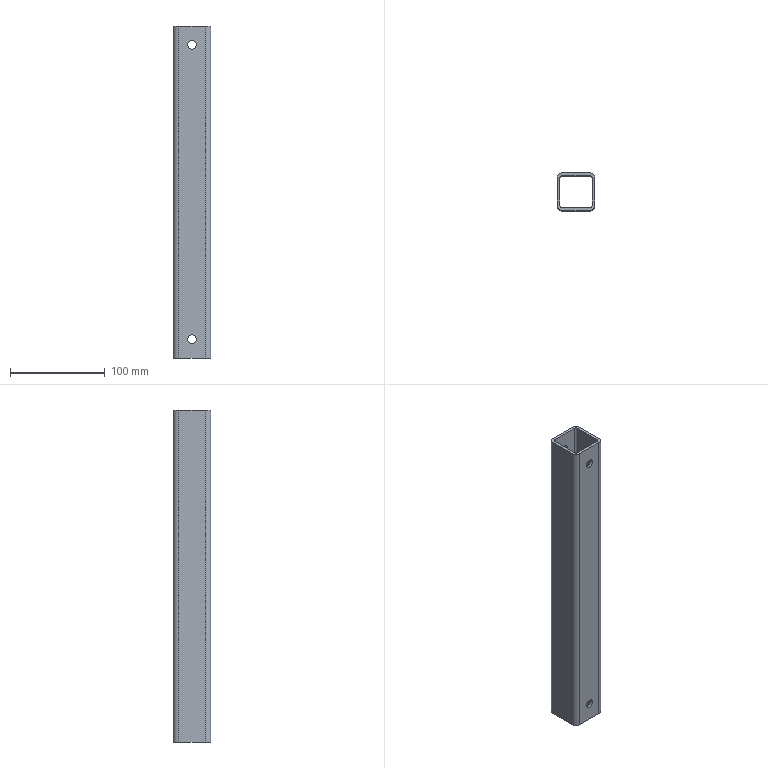Part | STEP file | DIN 59 410 - 40x40x2.9-400 | 1 solid | 22 faces | box 40 x 40 x 350 mm | volume 142308 mm3 | cylinder 12 | plane 10 | commonest cylinder face diameters 5.8 x4 9 x4 11.6 x4